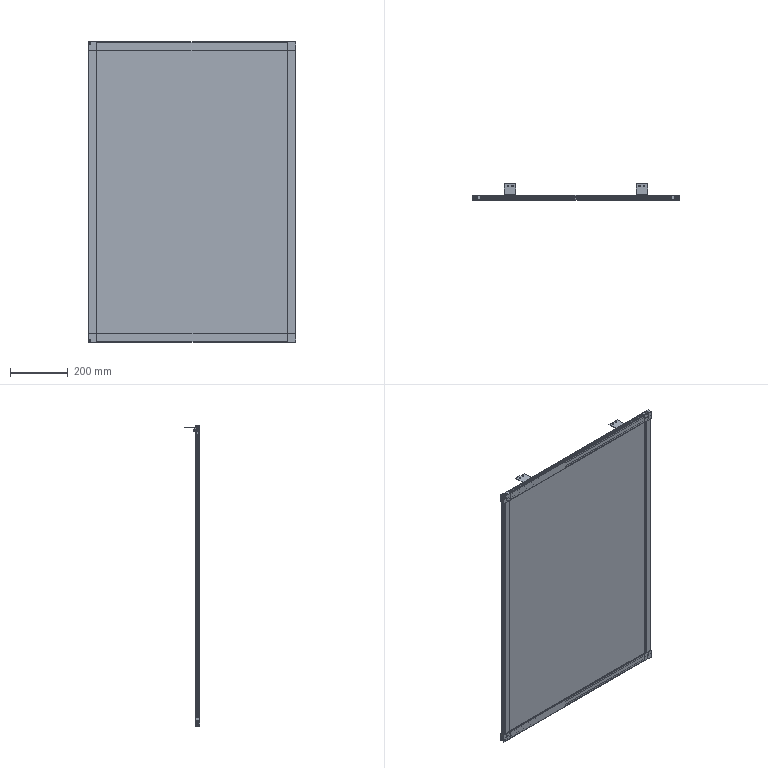Part | SolidWorks | features ReferencePattern 5, LocalLPattern 1 | 27 solids | 922 faces | box 722 x 54 x 1043 mm | volume 4219940 mm3 | plane 566 | cylinder 232 | cone 72 | spline 52 | commonest cylinder face diameters 11 x48 5 x44 1 x24 2 x16 3.3 x16 4.5 x16